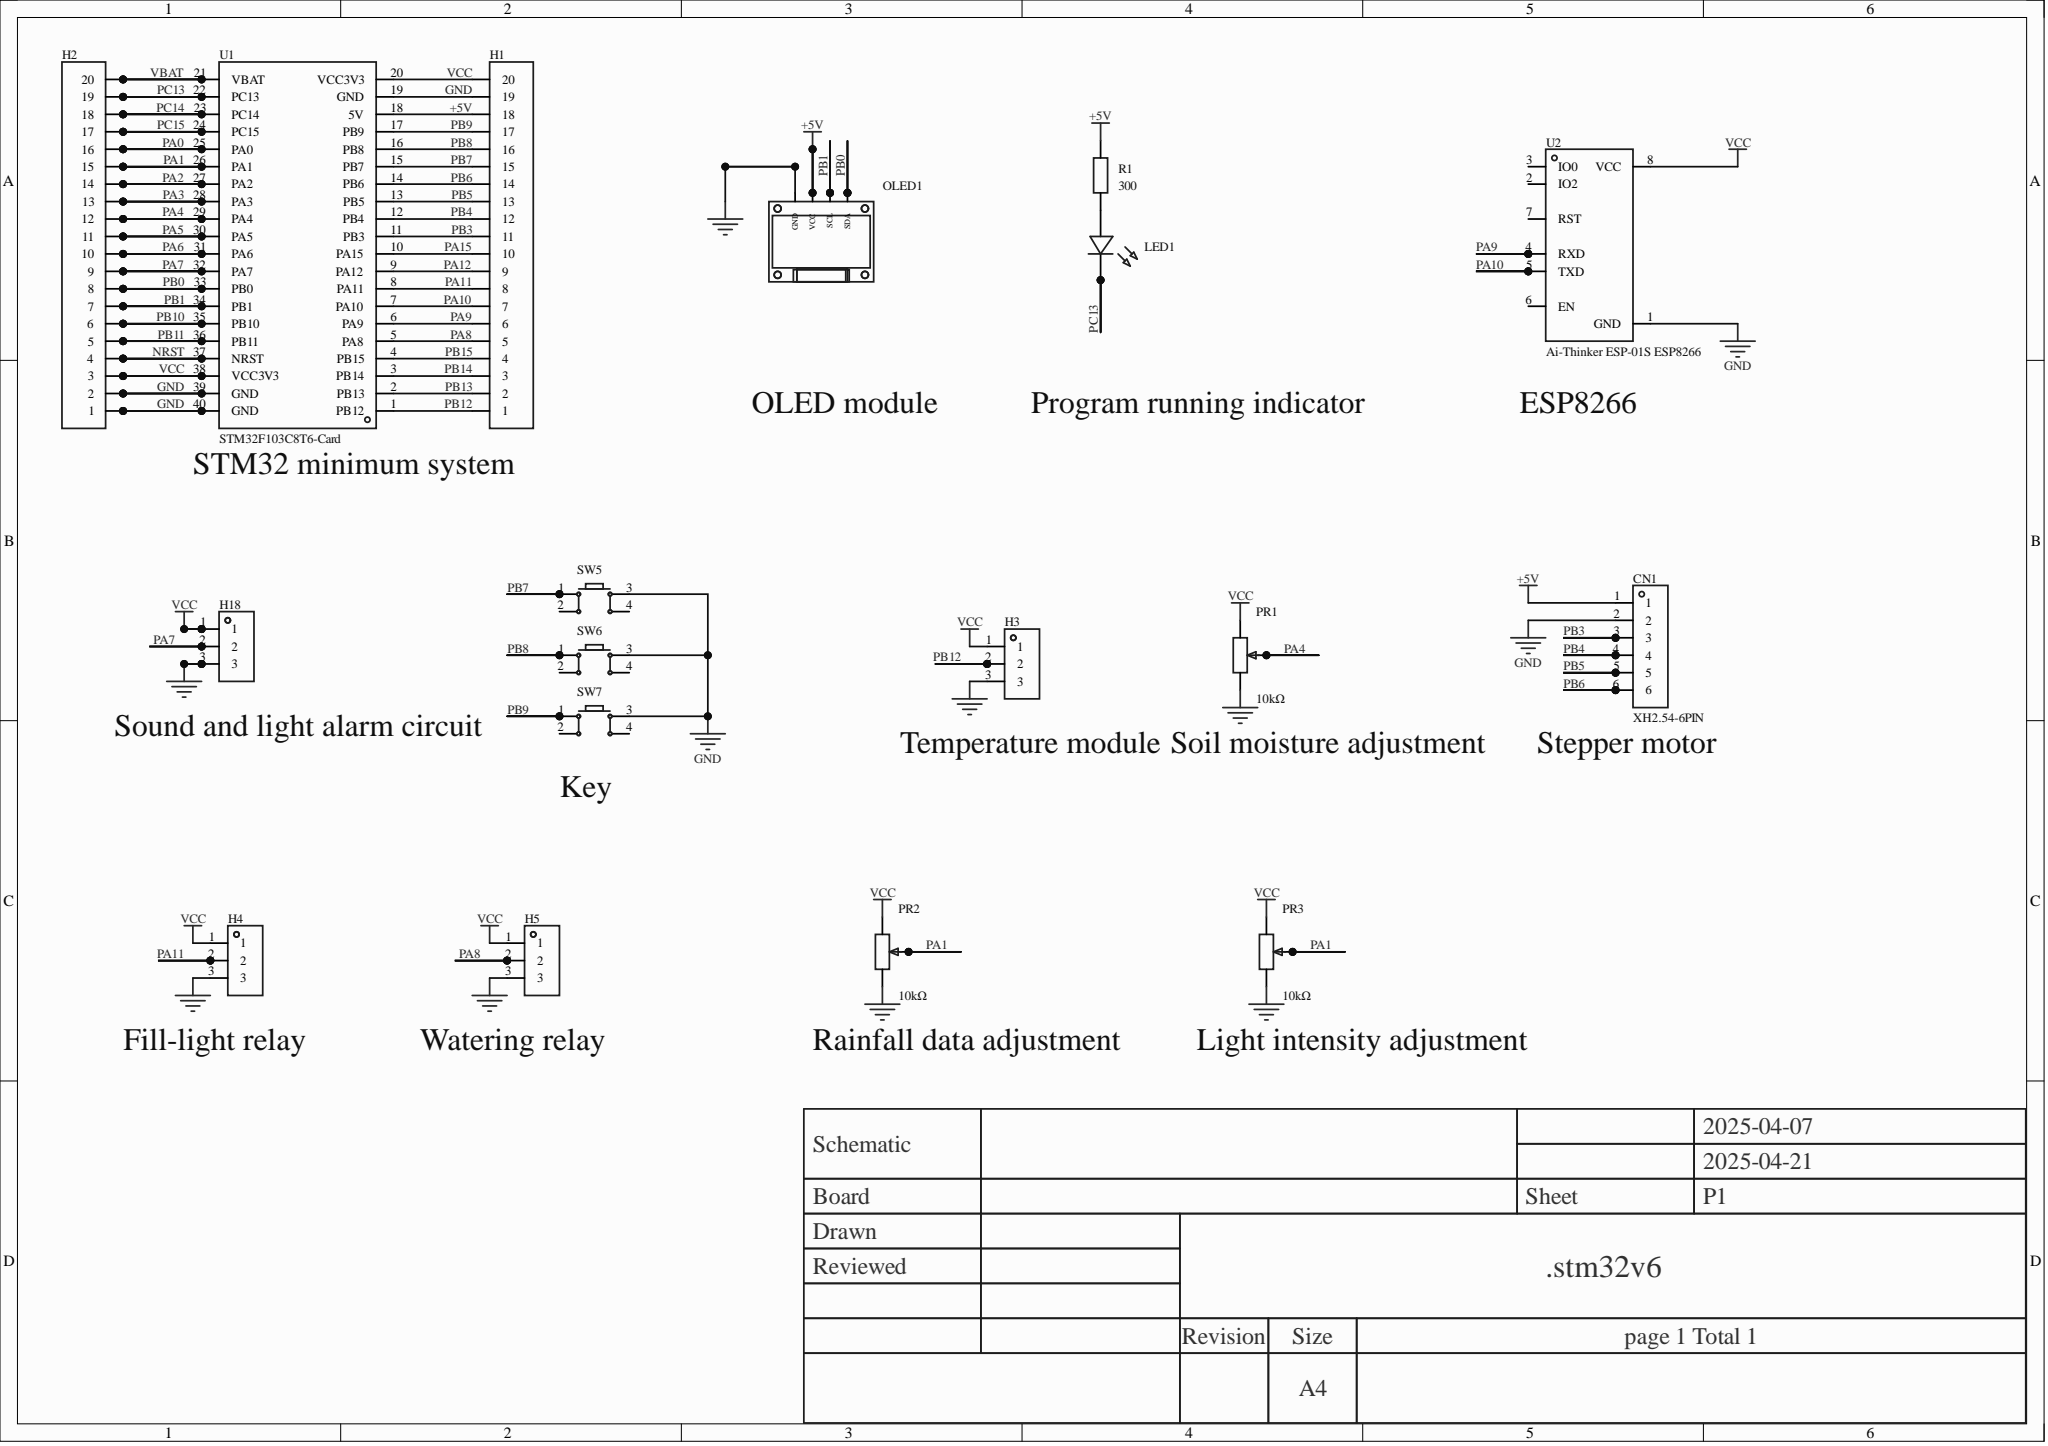Circuit board | Altium Designer | 18 parts | 38 nets
Bill of materials:
Comment,Description,Designator,Footprint,LibRef,Quantity
"XH2.54-6PIN","","CN1","CONN-TH_6P-P2.50-V-M_753","XH2.54-6PIN","1"
"","","H1, H2","HDR-TH_20P-P2.54-V-F","HDR-F_2.54_1x20P","2"
"","","H3, H4, H5, H18","HDR-TH_3P-P2.54-V-F","HDR-F_2.54_1x3P","4"
"","","LED1","LED_TH-3mm","LED_TH-R_3mm","1"
"","","OLED1","0.96OLED_4P","0.96OLED模块_4P","1"
"10kΩ","","PR1, PR2, PR3","R_3296","R_3296","3"
"300","","R1","R0603","Res_0603","1"
"","","SW5, SW6, SW7","SW-TH_4P-L6.0-W6.0-P4.50-LS6.5","Key_TH_6x6x6","3"
"STM32F103C8T6-Card","","U1","CONN-TH_L53.3-W22.9_STM32F103C8T6-CARD","STM32F103C8T6-Card","1"
"Ai-Thinker ESP-01S ESP8266","","U2","WIFIM-TH_8P-L24.7-W14.4-P2.54","Ai-Thinker ESP-01S ESP8266","1"
Netlist (Protel format):
[
CN1
CONN-TH_6P-P2.50-V-M_753
XH2.54-6PIN



]
[
H1
HDR-TH_20P-P2.54-V-F




]
[
H2
HDR-TH_20P-P2.54-V-F




]
[
H3
HDR-TH_3P-P2.54-V-F




]
[
H4
HDR-TH_3P-P2.54-V-F




]
[
H5
HDR-TH_3P-P2.54-V-F




]
[
H18
HDR-TH_3P-P2.54-V-F




]
[
LED1
LED_TH-3mm




]
[
OLED1
0.96OLED_4P




]
[
PR1
R_3296
10kΩ



]
[
PR2
R_3296
10kΩ



]
[
PR3
R_3296
10kΩ



]
[
R1
R0603
300



]
[
SW5
SW-TH_4P-L6.0-W6.0-P4.50-LS6.5




]
[
SW6
SW-TH_4P-L6.0-W6.0-P4.50-LS6.5




]
[
SW7
SW-TH_4P-L6.0-W6.0-P4.50-LS6.5




]
[
U1
CONN-TH_L53.3-W22.9_STM32F103C8T6-CARD
STM32F103C8T6-Card



]
[
U2
WIFIM-TH_8P-L24.7-W14.4-P2.54
Ai-Thinker ESP-01S ESP8266



]
(
VCC
H1-20
H2-3
H3-1
H4-1
H5-1
H18-1
PR1-3
PR2-3
PR3-3
U1-20
U1-38
U2-8
)
(
VBAT
H2-20
U1-21
)
(
PC15
H2-17
U1-24
)
(
PC14
H2-18
U1-23
)
(
PC13
H2-19
LED1-2
U1-22
)
(
PB15
H1-4
U1-4
)
(
PB14
H1-3
U1-3
)
(
PB13
H1-2
U1-2
)
(
PB12
H1-1
H3-2
U1-1
)
(
PB11
H2-5
U1-36
)
(
PB10
H2-6
U1-35
)
(
PB9
H1-17
SW7-1
U1-17
)
(
PB8
H1-16
SW6-1
U1-16
)
(
PB7
H1-15
SW5-1
U1-15
)
(
PB6
CN1-6
H1-14
U1-14
)
(
PB5
CN1-5
H1-13
U1-13
)
(
PB4
CN1-4
H1-12
U1-12
)
(
PB3
CN1-3
H1-11
U1-11
)
(
PB1
H2-7
OLED1-3
U1-34
)
(
PB0
H2-8
OLED1-4
U1-33
)
(
PA15
H1-10
U1-10
)
(
PA12
H1-9
U1-9
)
(
PA11
H1-8
H4-2
U1-8
)
(
PA10
H1-7
U1-7
U2-5
)
(
PA9
H1-6
U1-6
U2-4
)
(
PA8
H1-5
H5-2
U1-5
)
(
PA7
H2-9
H18-2
U1-32
)
(
PA6
H2-10
U1-31
)
(
PA5
H2-11
U1-30
)
(
PA4
H2-12
PR1-2
U1-29
)
(
PA3
H2-13
U1-28
)
(
PA2
H2-14
U1-27
)
(
PA1
H2-15
PR2-2
PR3-2
U1-26
)
(
PA0
H2-16
U1-25
)
(
NRST
H2-4
U1-37
)
(
NetLED1_1
LED1-1
R1-1
)
(
GND
CN1-2
H1-19
H2-1
H2-2
H3-3
H4-3
H5-3
H18-3
OLED1-1
PR1-1
PR2-1
PR3-1
SW5-3
SW6-3
SW7-3
U1-19
U1-39
U1-40
U2-1
)
(
+5V
CN1-1
H1-18
OLED1-2
R1-2
U1-18
)